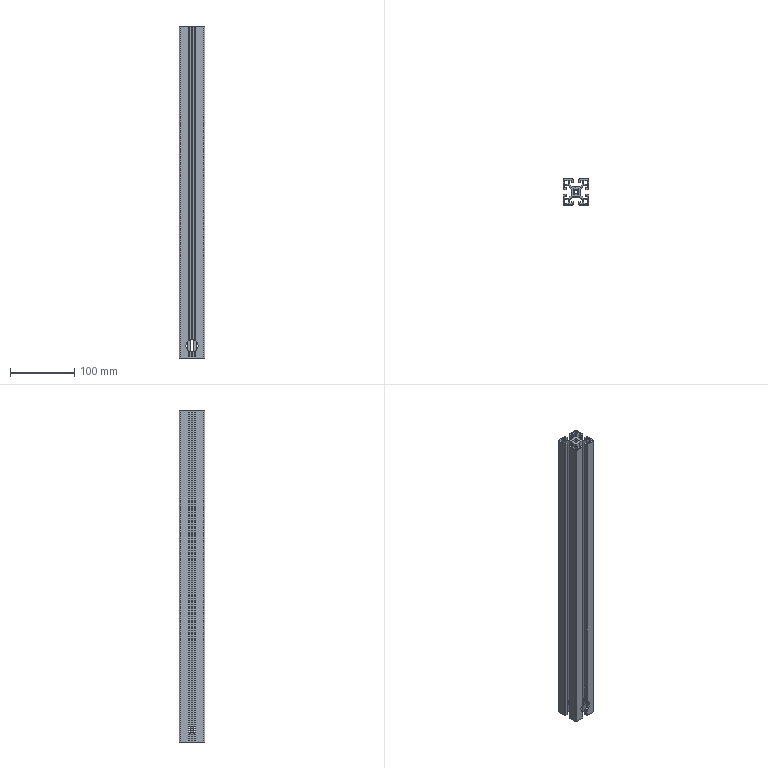Part | NX | features BREP 1 | 1 solid | 217 faces | box 40 x 40 x 515 mm | volume 309576 mm3 | plane 150 | cylinder 67 | commonest cylinder face diameters 0.6 x16 1.5 x12 2 x12 1 x8 19 x8 6.8 x7